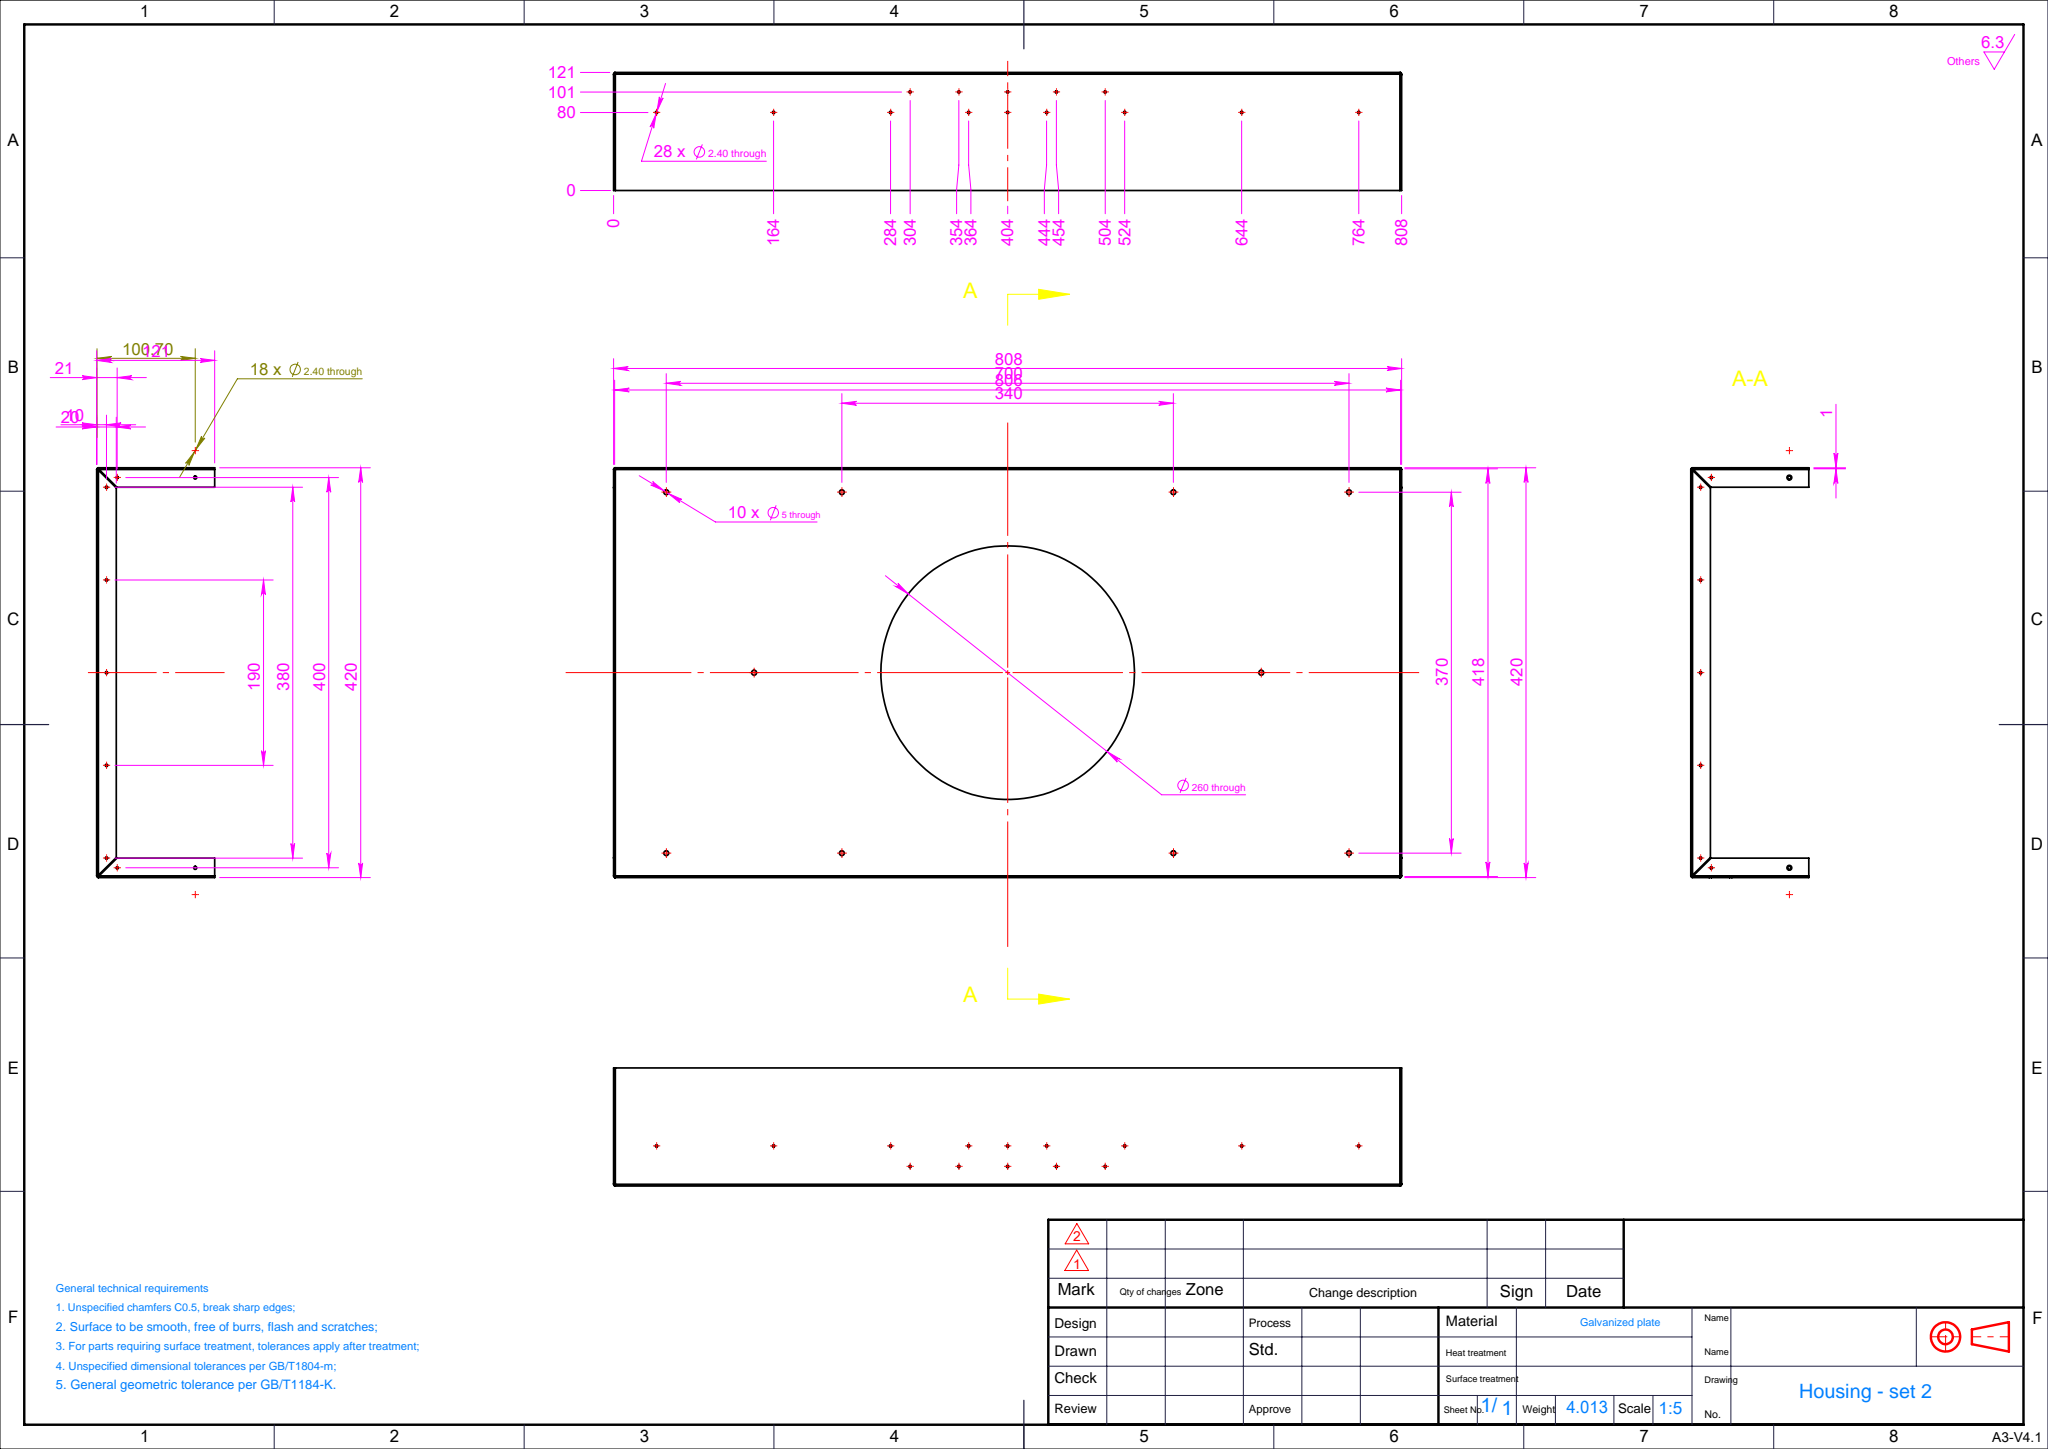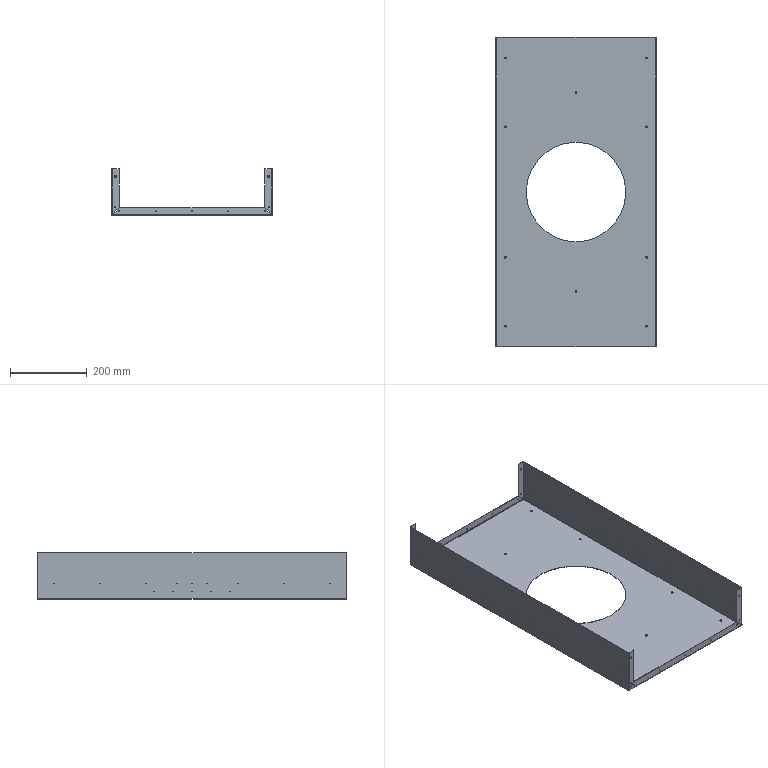Part | SolidWorks | features 3DProfileFeature 5, HoleWzd 5, SketchPattern 4, Chamfer 3, EdgeFlange 2, ICE 2, FlatPattern 1, SMBaseFlange 1, SheetMetal 1 | 1 solid | 200 faces | box 420 x 808 x 121 mm | volume 501647 mm3 | cylinder 130 | plane 54 | cone 8 | spline 8 | commonest cylinder face diameters 2.4 x84 5 x20 1.473 x8 3.2 x8 3.473 x8 260 x2